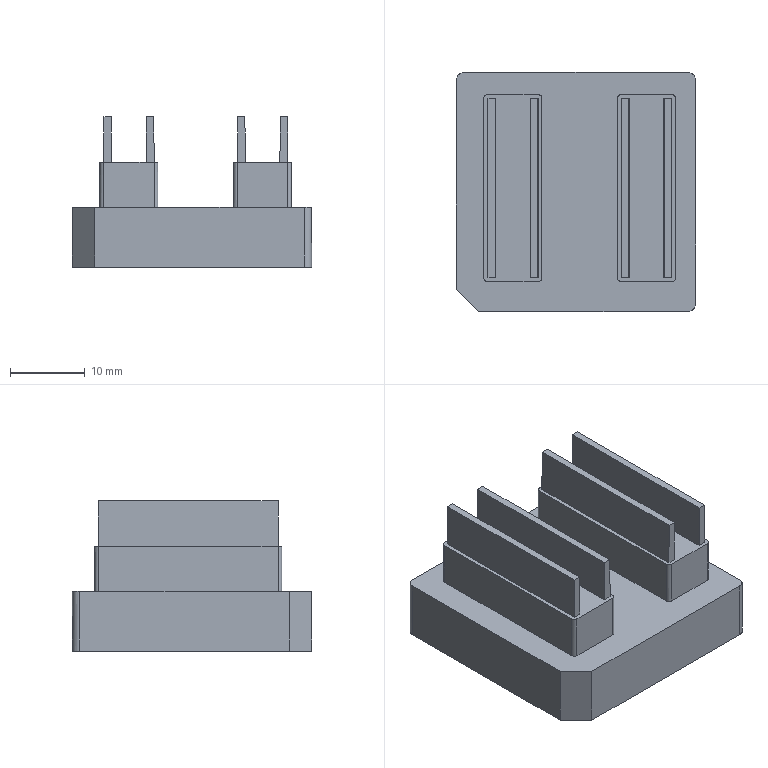NC program | PowerMill | posted with a generic post | part box 32 x 32 x 20.109 mm
Lines 17639 to 18576 of 124326:
N17736 M6
N17737 S8500 M03
N17738 G00 G90 X0.0 Y0.0
N17739 G43 Z11.799 H3
N17740
N17741 G05 P10000 R8
N17742 X15.0099 Y-22.0332
N17743 Z0.9292
N17744 G01 Z-0.2708 F360.0
N17745 X13.9138 Y-16.8733 F600.0
N17746 X13.82 Y17.8929
N17747 X13.5596 Y17.9372
N17748 X13.3468 Y17.9633
N17749 X13.1156 Y17.9827
N17750 X12.8038 Y17.9934
N17751 X11.7079 Y17.9924
N17752 X11.4173 Y17.9789
N17753 X11.2092 Y17.9599
N17754 X11.0271 Y17.9367
N17755 X10.8474 Y17.9075
N17756 X10.562 Y17.8485
N17757 X10.2766 Y17.7734
N17758 X9.9964 Y17.6832
N17759 X9.7057 Y17.5716
N17760 X9.4461 Y17.4547
N17761 X9.3999 Y17.477
N17762 X9.4915 Y-16.4749
N17763 X9.4468 Y-16.4548
N17764 X9.2705 Y-16.5356
N17765 X9.0907 Y-16.6079
N17766 G02 X8.6522 Y-16.7622 I-1.6733 J4.0563
N17767 G01 X8.3857 Y-16.8343
N17768 X8.0819 Y-16.9006
N17769 X7.8594 Y-16.9374
N17770 X7.5105 Y-16.9761
N17771 X7.2257 Y-16.9912
N17772 X6.1649 Y-16.9935
N17773 X5.826 Y-16.9853
N17774 X5.5717 Y-16.9665
N17775 X5.2196 Y-16.9201
N17776 X5.0713 Y-16.892
N17777 X4.9775 Y17.8737
N17778 G00 Z3.9992
N17779 G01 X-3.0555 Y-22.0678 F10000.0
N17780 G00 Z0.9292
N17781 G01 Z-0.2708 F360.0
N17782 X-4.0258 Y-16.8828 F600.0
N17783 X-4.0473 Y17.8862
N17784 X-4.3285 Y17.9368
N17785 G03 X-4.8989 Y17.9892 I-0.8406 J-6.0212
N17786 G01 X-5.2165 Y17.9935
N17787 X-6.2303 Y17.9911
N17788 X-6.5074 Y17.9761
N17789 X-6.8647 Y17.9366
N17790 X-7.0865 Y17.8997
N17791 X-7.3668 Y17.8396
N17792 X-7.6574 Y17.7606
N17793 G03 X-8.4454 Y17.455 I1.6281 J-5.367
N17794 G01 X-8.4559 Y17.4602
N17795 X-8.435 Y-16.4601
N17796 X-8.4457 Y-16.4552
N17797 X-8.711 Y-16.5739
N17798 X-8.9966 Y-16.6831
N17799 X-9.2973 Y-16.779
N17800 X-9.5621 Y-16.8483
N17801 X-9.7937 Y-16.897
N17802 X-10.0271 Y-16.9367
N17803 X-10.2617 Y-16.9654
N17804 X-10.4825 Y-16.9825
N17805 X-10.7037 Y-16.9922
N17806 X-11.8599 Y-16.9928
N17807 X-12.1111 Y-16.983
N17808 X-12.3358 Y-16.9645
N17809 X-12.563 Y-16.9367
N17810 X-12.8437 Y-16.8882
N17811 X-12.8651 Y17.8823
N17812 G00 Z11.799
N17813 G05 P0
N17814 (---------------)
N17815 ( END TOOLPATH : 精公基准台01-平坦面平行-D10 )
N17816 (---------------)
N17817 ( START TOOLPATH : 精公基准台01-基准面偏置-D10 )
N17818 (---------------)
N17819 G00 X0.0 Y0.0 Z9.7992
N17820 G05 P10000 R8
N17821 X26.755 Y-4.9778
N17822 Z-11.11
N17823 G01 Z-12.31 F360.0
N17824 X21.48 F600.0
N17825 X18.7097 Y0.5627
N17826 Y-11.2546
N17827 X18.7014 Y-11.8173
N17828 X18.6806 Y-12.0987
N17829 X18.6457 Y-12.3801
N17830 X18.5701 Y-12.7867
N17831 X18.5333 Y-12.9428
N17832 X18.4555 Y-13.2242
N17833 X18.3621 Y-13.5055
N17834 X18.2525 Y-13.7869
N17835 X18.1258 Y-14.0683
N17836 X18.0074 Y-14.3002
N17837 X17.815 Y-14.631
N17838 X17.6412 Y-14.8938
N17839 X17.415 Y-15.1937
N17840 X17.1741 Y-15.4751
N17841 X17.0423 Y-15.6158
N17842 X16.8819 Y-15.774
N17843 X16.6005 Y-16.0251
N17844 X16.3192 Y-16.2464
N17845 X16.2181 Y-16.3192
N17846 X15.9873 Y-16.4738
N17847 X15.7565 Y-16.6135
N17848 X15.4903 Y-16.7573
N17849 X15.1937 Y-16.8973
N17850 X14.9124 Y-17.0124
N17851 X14.631 Y-17.1108
N17852 X14.3496 Y-17.1933
N17853 X14.0683 Y-17.2616
N17854 X13.7869 Y-17.3151
N17855 X13.5055 Y-17.3545
N17856 X13.2242 Y-17.3791
N17857 X12.9428 Y-17.3924
N17858 X5.9087 Y-17.3915
N17859 X5.6273 Y-17.3773
N17860 X5.3459 Y-17.35
N17861 X5.0646 Y-17.3084
N17862 X4.7832 Y-17.2529
N17863 X4.5018 Y-17.1831
N17864 X4.2205 Y-17.098
N17865 X3.9391 Y-16.997
N17866 X3.663 Y-16.8819
N17867 X3.3764 Y-16.7448
N17868 X3.095 Y-16.5896
N17869 X2.8137 Y-16.4154
N17870 X2.6732 Y-16.3192
N17871 X2.4621 Y-16.1629
N17872 X2.2509 Y-15.9897
N17873 X1.9907 Y-15.7565
N17874 X1.8334 Y-15.5998
N17875 X1.6882 Y-15.4432
N17876 X1.4755 Y-15.1937
N17877 X1.2946 Y-14.9562
N17878 G03 X-0.2981 Y-14.9582 I-0.7956 J-0.6059
N17879 G01 X-0.4765 Y-15.1937
N17880 X-0.5627 Y-15.2976
N17881 X-0.7639 Y-15.5262
N17882 X-0.9908 Y-15.7565
N17883 X-1.1255 Y-15.8812
N17884 X-1.4001 Y-16.1145
N17885 X-1.6882 Y-16.3296
N17886 X-1.9696 Y-16.515
N17887 X-2.2509 Y-16.6783
N17888 X-2.4582 Y-16.7861
N17889 X-2.6625 Y-16.8819
N17890 X-2.8137 Y-16.947
N17891 X-3.095 Y-17.0551
N17892 X-3.3764 Y-17.1471
N17893 X-3.6577 Y-17.2231
N17894 X-3.9391 Y-17.2856
N17895 X-4.2205 Y-17.333
N17896 X-4.5018 Y-17.3663
N17897 X-4.7832 Y-17.3863
N17898 X-5.0646 Y-17.3935
N17899 X-11.8173
N17900 X-12.0987 Y-17.3869
N17901 X-12.3801 Y-17.3677
N17902 X-12.6614 Y-17.3346
N17903 X-12.9428 Y-17.2872
N17904 X-13.2242 Y-17.2259
N17905 X-13.5055 Y-17.1498
N17906 X-13.7869 Y-17.0582
N17907 X-14.0683 Y-16.9509
N17908 X-14.2496 Y-16.8724
N17909 X-14.4284 Y-16.7883
N17910 X-14.631 Y-16.6833
N17911 X-14.9124 Y-16.5204
N17912 X-15.2179 Y-16.3192
N17913 X-15.4872 Y-16.117
N17914 X-15.7565 Y-15.8892
N17915 X-15.9004 Y-15.7565
N17916 X-16.1203 Y-15.5336
N17917 X-16.3192 Y-15.3108
N17918 X-16.4156 Y-15.1937
N17919 X-16.628 Y-14.9124
N17920 X-16.8154 Y-14.631
N17921 X-16.8819 Y-14.5216
N17922 X-17.0104 Y-14.2949
N17923 X-17.1259 Y-14.0683
N17924 X-17.2526 Y-13.7869
N17925 X-17.3622 Y-13.5055
N17926 X-17.4446 Y-13.2591
N17927 X-17.5328 Y-12.9428
N17928 X-17.5967 Y-12.6614
N17929 X-17.6455 Y-12.3801
N17930 X-17.68 Y-12.0987
N17931 X-17.7013 Y-11.8173
N17932 X-17.7098 Y-11.2546
N17933 X-17.7077 Y12.6614
N17934 X-17.6939 Y12.9428
N17935 X-17.6667 Y13.2242
N17936 X-17.6254 Y13.5055
N17937 X-17.5702 Y13.7869
N17938 X-17.5004 Y14.0683
N17939 X-17.4446 Y14.259
N17940 X-17.3152 Y14.631
N17941 X-17.1982 Y14.9124
N17942 X-17.0635 Y15.1937
N17943 X-16.8819 Y15.5204
N17944 X-16.7346 Y15.7565
N17945 X-16.5405 Y16.0325
N17946 X-16.3101 Y16.3192
N17947 X-16.0571 Y16.6005
N17948 X-15.911 Y16.7466
N17949 X-15.7565 Y16.8896
N17950 X-15.4751 Y17.1273
N17951 X-15.1937 Y17.3361
N17952 X-15.0324 Y17.4446
N17953 X-14.8317 Y17.5697
N17954 X-14.631 Y17.6834
N17955 X-14.3496 Y17.8262
N17956 X-14.0683 Y17.9508
N17957 X-13.9251 Y18.0074
N17958 X-13.5055 Y18.1497
N17959 X-13.2242 Y18.2253
N17960 X-12.9428 Y18.2874
N17961 X-12.6614 Y18.3346
N17962 X-12.3801 Y18.3671
N17963 X-12.0987 Y18.3871
N17964 X-11.8173 Y18.3937
N17965 X-5.0646
N17966 X-4.7832 Y18.3867
N17967 X-4.5018 Y18.3671
N17968 X-4.2205 Y18.3332
N17969 X-3.9391 Y18.2854
N17970 X-3.6577 Y18.2235
N17971 X-3.3764 Y18.147
N17972 X-2.9659 Y18.0074
N17973 X-2.8137 Y17.9469
N17974 X-2.5323 Y17.8218
N17975 X-2.2509 Y17.6782
N17976 X-1.8585 Y17.4446
N17977 X-1.6882 Y17.3298
N17978 X-1.4081 Y17.1203
N17979 X-1.1255 Y16.8808
N17980 X-0.98 Y16.7462
N17981 X-0.8331 Y16.5995
N17982 X-0.5627 Y16.2997
N17983 X-0.3183 Y15.9869
N17984 G03 X1.3179 Y15.9858 I0.8185 J0.5745
N17985 G01 X1.3545 Y16.0378
N17986 X1.581 Y16.3192
N17987 X1.6882 Y16.4428
N17988 X1.8941 Y16.6617
N17989 X2.1265 Y16.8819
N17990 X2.2509 Y16.9915
N17991 X2.5323 Y17.2168
N17992 X2.8587 Y17.4446
N17993 X3.1175 Y17.6035
N17994 X3.3764 Y17.7447
N17995 X3.6582 Y17.8799
N17996 X3.966 Y18.0074
N17997 X4.2339 Y18.1024
N17998 X4.5018 Y18.1827
N17999 X4.7832 Y18.2528
N18000 X5.0646 Y18.3085
N18001 X5.3459 Y18.3496
N18002 X5.6273 Y18.3761
N18003 X5.9087 Y18.3917
N18004 X12.9428 Y18.3923
N18005 X13.2242 Y18.3801
N18006 X13.5055 Y18.3547
N18007 X13.7869 Y18.3153
N18008 X14.0683 Y18.2615
N18009 X14.3496 Y18.1939
N18010 X14.631 Y18.111
N18011 X14.9257 Y18.0074
N18012 X15.1937 Y17.8972
N18013 X15.4751 Y17.7651
N18014 X15.7565 Y17.6128
N18015 X16.0326 Y17.4446
N18016 X16.3192 Y17.2463
N18017 X16.5412 Y17.0731
N18018 X16.7646 Y16.8819
N18019 X16.8819 Y16.7742
N18020 X17.1089 Y16.546
N18021 X17.3119 Y16.3192
N18022 X17.4446 Y16.1573
N18023 X17.5971 Y15.9557
N18024 X17.7345 Y15.7565
N18025 X17.8791 Y15.5267
N18026 X18.0074 Y15.3003
N18027 X18.0634 Y15.1937
N18028 X18.1982 Y14.9124
N18029 X18.3151 Y14.631
N18030 X18.4159 Y14.3496
N18031 X18.5003 Y14.0683
N18032 X18.5701 Y13.7863
N18033 X18.6253 Y13.5055
N18034 X18.6665 Y13.2242
N18035 X18.6927 Y12.9428
N18036 X18.7078 Y12.6614
N18037 X18.7097 Y0.5627
N18038 G00 Z9.7992
N18039 G05 P0
N18040 (---------------)
N18041 ( END TOOLPATH : 精公基准台01-基准面偏置-D10 )
N18042 (---------------)
N18043 ( START TOOLPATH : 精公基准台01-外形侧光-D10 )
N18044 (---------------)
N18045 G00 X0.0 Y0.0 Z10.799
N18046 G05 P10000 R8
N18047 X0.5029 Y-13.8692
N18048 Z-11.08
N18049 G01 Z-12.28 F360.0
N18050 G03 X-0.4439 Y-14.5185 I0.3104 J-1.4675 F600.0
N18051 G02 X-5.1116 Y-17.0235 I-4.6196 J3.0068
N18052 G01 X-8.447 Y-17.0234
N18053 X-11.8682 Y-17.0233
N18054 G02 X-17.3397 Y-11.501 I0.0399 J5.5112
N18055 G01 X-17.3393 Y0.4564
N18056 X-17.3389 Y12.5992
N18057 G02 X-11.8662 Y18.0234 I5.5106 J-0.0871
N18058 G01 X-5.1108 Y18.0235
N18059 G02 X0.4478 Y12.5964 I0.047 J-5.512
N18060 G01 X0.4485 Y-11.5023
N18061 G02 X-0.4439 Y-14.5185 I-5.512 J-0.0094
N18062 G03 X-0.6542 Y-15.6471 I1.2572 J-0.8182
N18063 G01 X0.4545 Y-13.781
N18064 G03 X-0.4871 Y-14.4379 I0.3222 J-1.465
N18065 G02 X-5.1116 Y-16.9435 I-4.5764 J2.9262
N18066 G01 X-8.447 Y-16.9434
N18067 X-11.8662
N18068 G02 X-17.2597 Y-11.501 I0.0379 J5.4313
N18069 G01 Y0.4564
N18070 Y12.4138
N18071 G02 X-11.8662 Y17.9434 I5.4334 J0.0955
N18072 G01 X-5.1116 Y17.9435
N18073 G02 X0.3685 Y12.4138 I0.0458 J-5.4349
N18074 G01 Y-11.501
N18075 G02 X-0.4871 Y-14.4379 I-5.432 J-0.0107
N18076 G03 X-0.6883 Y-15.5682 I1.2638 J-0.8081
N18077 G00 Z3.9551
N18078 G01 X18.407 Y-13.8387 F10000.0
N18079 G00 Z-11.08
N18080 G01 Z-12.28 F360.0
N18081 G03 X17.4637 Y-14.4932 I0.3184 J-1.4658 F600.0
N18082 G02 X12.7789 Y-17.0235 I-4.636 J2.9815
N18083 G01 X6.0223 Y-17.0233
N18084 G02 X0.5515 Y-11.501 I0.0406 J5.5112
N18085 G01 X0.5519 Y0.4564
N18086 X0.5523 Y12.5992
N18087 G02 X1.2792 Y15.2491 I5.5107 J-0.0871
N18088 G02 X6.0244 Y18.0234 I4.7837 J-2.737
N18089 G01 X12.7797 Y18.0235
N18090 G02 X18.339 Y12.5964 I0.048 J-5.5118
N18091 G01 X18.3397 Y-11.5023
N18092 G02 X17.4637 Y-14.4932 I-5.512 J-0.0094
N18093 G03 X17.2595 Y-15.6229 I1.2617 J-0.8113
N18094 G01 X18.3581 Y-13.7505
N18095 G03 X17.4202 Y-14.4126 I0.3303 J-1.4632
N18096 G02 X12.7789 Y-16.9435 I-4.5925 J2.9009
N18097 G01 X6.0244 Y-16.9434
N18098 G02 X0.6315 Y-11.501 I0.0385 J5.4313
N18099 G01 Y0.4564
N18100 Y12.4138
N18101 G02 X1.3489 Y15.2092 I5.4334 J0.0955
N18102 G02 X6.0244 Y17.9434 I4.716 J-2.6999
N18103 G01 X12.7789 Y17.9435
N18104 G02 X18.2597 Y12.4138 I0.0469 J-5.4345
N18105 G01 Y-11.501
N18106 G02 X17.4202 Y-14.4126 I-5.432 J-0.0107
N18107 G03 X17.2252 Y-15.544 I1.2682 J-0.8011
N18108 G00 Z10.799
N18109 G05 P0
N18110 (---------------)
N18111 ( END TOOLPATH : 精公基准台01-外形侧光-D10 )
N18112 (---------------)
N18113 ( START TOOLPATH : 精公基准台01-基准台侧光-D10 )
N18114 (---------------)
N18115 G00 X0.0 Y0.0 Z9.7992
N18116 G05 P10000 R8
N18117 X21.439 Y-24.0159
N18118 Z-19.01
N18119 G01 Z-20.21 F360.0
N18120 G03 X18.4869 Y-19.9804 I-1.476 J2.0177 F600.0
N18121 G01 X18.4851 Y-19.9817
N18122 X18.4839 Y-19.9826
N18123 X18.4827 Y-19.9835
N18124 X18.3812 Y-20.052
N18125 X18.3801 Y-20.0527
N18126 X18.379 Y-20.0535
N18127 X18.0629 Y-20.2521
N18128 X18.0607 Y-20.2534
N18129 X18.0585 Y-20.2547
N18130 X17.7423 Y-20.4263
N18131 X17.7402 Y-20.4274
N18132 X17.7381 Y-20.4285
N18133 X17.422 Y-20.5767
N18134 X17.4199 Y-20.5776
N18135 X17.4178 Y-20.5785
N18136 X17.1016 Y-20.7052
N18137 X17.0995 Y-20.706
N18138 X17.0974 Y-20.7067
N18139 X16.7812 Y-20.8131
N18140 X16.7791 Y-20.8138
N18141 X16.777 Y-20.8144
N18142 X16.4609 Y-20.9018
N18143 X16.4593 Y-20.9022
N18144 X16.4576 Y-20.9026
N18145 X16.2808 Y-20.9435
N18146 X16.2797 Y-20.9438
N18147 X16.2785 Y-20.944
N18148 X16.1392 Y-20.9721
N18149 X16.1378 Y-20.9723
N18150 X16.1364 Y-20.9726
N18151 X15.8202 Y-21.0244
N18152 X15.8181 Y-21.0247
N18153 X15.8159 Y-21.025
N18154 X15.4997 Y-21.0591
N18155 X15.4976 Y-21.0593
N18156 X15.4955 Y-21.0595
N18157 X15.1794 Y-21.0768
N18158 X15.1776 Y-21.0769
N18159 X15.1758
N18160 X14.8596 Y-21.08
N18161 X14.8592
N18162 X14.8588
N18163 X-12.962
N18164 X-12.963
N18165 X-12.9639
N18166 X-13.2801 Y-21.0722
N18167 X-13.2826 Y-21.0721
N18168 X-13.2851 Y-21.072
N18169 X-13.6012 Y-21.0443
N18170 X-13.6038 Y-21.044
N18171 X-13.6063 Y-21.0436
N18172 X-13.9224 Y-20.9955
N18173 X-13.925 Y-20.9951
N18174 X-13.9275 Y-20.9946
N18175 X-14.2437 Y-20.9254
N18176 X-14.2462 Y-20.9248
N18177 X-14.2487 Y-20.9241
N18178 X-14.5649 Y-20.8329
N18179 X-14.5674 Y-20.8322
N18180 X-14.5699 Y-20.8313
N18181 X-14.8861 Y-20.7169
N18182 X-14.8882 Y-20.7161
N18183 X-14.8903 Y-20.7152
N18184 X-15.1057 Y-20.623
N18185 X-15.107 Y-20.6225
N18186 X-15.1082 Y-20.6219
N18187 X-15.209 Y-20.5746
N18188 X-15.2107 Y-20.5738
N18189 X-15.2123 Y-20.5729
N18190 X-15.5285 Y-20.406
N18191 X-15.5304 Y-20.4049
N18192 X-15.5324 Y-20.4038
N18193 X-15.7019 Y-20.3019
N18194 X-15.7031 Y-20.3011
N18195 X-15.7044 Y-20.3003
N18196 X-15.851 Y-20.2045
N18197 X-15.8529 Y-20.2033
N18198 X-15.8546 Y-20.202
N18199 X-16.1547 Y-19.9817
N18200 X-16.1573 Y-19.9797
N18201 X-16.1598 Y-19.9776
N18202 X-16.492 Y-19.6894
N18203 X-16.494 Y-19.6876
N18204 X-16.4959 Y-19.6858
N18205 X-16.8121 Y-19.3722
N18206 X-16.8122 Y-19.372
N18207 X-16.8123 Y-19.3719
N18208 X-19.6576 Y-16.5254
N18209 X-19.6594 Y-16.5235
N18210 X-19.6611 Y-16.5216
N18211 X-19.9645 Y-16.1762
N18212 X-19.9667 Y-16.1736
N18213 X-19.9688 Y-16.1709
N18214 X-20.2019 Y-15.8548
N18215 X-20.2032 Y-15.8529
N18216 X-20.2045 Y-15.851
N18217 X-20.3003 Y-15.7044
N18218 X-20.3011 Y-15.7031
N18219 X-20.3019 Y-15.7019
N18220 X-20.4038 Y-15.5324
N18221 X-20.4049 Y-15.5304
N18222 X-20.406 Y-15.5285
N18223 X-20.5729 Y-15.2123
N18224 X-20.5738 Y-15.2107
N18225 X-20.5746 Y-15.209
N18226 X-20.6219 Y-15.1082
N18227 X-20.6225 Y-15.107
N18228 X-20.623 Y-15.1057
N18229 X-20.7152 Y-14.8903
N18230 X-20.7161 Y-14.8882
N18231 X-20.7169 Y-14.8861
N18232 X-20.8313 Y-14.5699
N18233 X-20.8322 Y-14.5674
N18234 X-20.8329 Y-14.5649
N18235 X-20.9241 Y-14.2487
N18236 X-20.9248 Y-14.2462
N18237 X-20.9254 Y-14.2437
N18238 X-20.9946 Y-13.9275
N18239 X-20.9951 Y-13.925
N18240 X-20.9955 Y-13.9224
N18241 X-21.0436 Y-13.6063
N18242 X-21.044 Y-13.6038
N18243 X-21.0443 Y-13.6012
N18244 X-21.072 Y-13.2851
N18245 X-21.0721 Y-13.2826
N18246 X-21.0722 Y-13.2801
N18247 X-21.08 Y-12.9639
N18248 Y-12.963
N18249 Y-12.962
N18250 Y14.8588
N18251 Y14.8592
N18252 Y14.8596
N18253 X-21.077 Y15.1758
N18254 X-21.0769 Y15.1775
N18255 X-21.0768 Y15.1793
N18256 X-21.0597 Y15.4955
N18257 X-21.0596 Y15.4976
N18258 X-21.0594 Y15.4998
N18259 X-21.025 Y15.8159
N18260 X-21.0247 Y15.8181
N18261 X-21.0244 Y15.8202
N18262 X-20.9728 Y16.1363
N18263 X-20.9724 Y16.1384
N18264 X-20.972 Y16.1405
N18265 X-20.9029 Y16.4567
N18266 X-20.9024 Y16.4588
N18267 X-20.9018 Y16.4609
N18268 X-20.8145 Y16.777
N18269 X-20.8139 Y16.7792
N18270 X-20.8131 Y16.7814
N18271 X-20.706 Y17.0975
N18272 X-20.7053 Y17.0995
N18273 X-20.7046 Y17.1015
N18274 X-20.5786 Y17.4176
N18275 X-20.5776 Y17.4199
N18276 X-20.5766 Y17.4221
N18277 X-20.4277 Y17.7383
N18278 X-20.4267 Y17.7402
N18279 X-20.4257 Y17.7422
N18280 X-20.2547 Y18.0584
N18281 X-20.2535 Y18.0605
N18282 X-20.2522 Y18.0627
N18283 X-20.0546 Y18.3788
N18284 X-20.0537 Y18.3802
N18285 X-20.0528 Y18.3816
N18286 X-19.9832 Y18.4834
N18287 X-19.9825 Y18.4845
N18288 X-19.9817 Y18.4855
N18289 X-19.8246 Y18.6999
N18290 X-19.8236 Y18.7013
N18291 X-19.8225 Y18.7026
N18292 X-19.6635 Y18.9011
N18293 X-19.6626 Y18.9021
N18294 X-19.6617 Y18.9032
N18295 X-19.5606 Y19.0209
N18296 X-19.5595 Y19.0221
N18297 X-19.5585 Y19.0232
N18298 X-19.3435 Y19.2544
N18299 X-19.3425 Y19.2554
N18300 X-19.3415 Y19.2565
N18301 X-19.2565 Y19.3415
N18302 X-19.2554 Y19.3425
N18303 X-19.2544 Y19.3435
N18304 X-19.0232 Y19.5584
N18305 X-19.022 Y19.5596
N18306 X-19.0207 Y19.5607
N18307 X-18.9022 Y19.6619
N18308 X-18.9013 Y19.6626
N18309 X-18.9004 Y19.6634
N18310 X-18.7028 Y19.8224
N18311 X-18.7013 Y19.8236
N18312 X-18.6998 Y19.8247
N18313 X-18.4851 Y19.9817
N18314 X-18.4839 Y19.9826
N18315 X-18.4827 Y19.9835
N18316 X-18.3812 Y20.052
N18317 X-18.3801 Y20.0527
N18318 X-18.379 Y20.0535
N18319 X-18.0629 Y20.2521
N18320 X-18.0607 Y20.2534
N18321 X-18.0585 Y20.2547
N18322 X-17.7423 Y20.4263
N18323 X-17.7402 Y20.4274
N18324 X-17.7381 Y20.4285
N18325 X-17.422 Y20.5767
N18326 X-17.4199 Y20.5776
N18327 X-17.4178 Y20.5785
N18328 X-17.1016 Y20.7052
N18329 X-17.0995 Y20.706
N18330 X-17.0974 Y20.7067
N18331 X-16.7812 Y20.8131
N18332 X-16.7791 Y20.8138
N18333 X-16.777 Y20.8144
N18334 X-16.4609 Y20.9018
N18335 X-16.4588 Y20.9023
N18336 X-16.4566 Y20.9028
N18337 X-16.1405 Y20.9718
N18338 X-16.1384 Y20.9722
N18339 X-16.1364 Y20.9726
N18340 X-15.8202 Y21.0244
N18341 X-15.8181 Y21.0247
N18342 X-15.8159 Y21.025
N18343 X-15.4997 Y21.0591
N18344 X-15.4976 Y21.0593
N18345 X-15.4955 Y21.0595
N18346 X-15.1794 Y21.0768
N18347 X-15.1776 Y21.0769
N18348 X-15.1758
N18349 X-14.8596 Y21.08
N18350 X-14.8592
N18351 X-14.8588
N18352 X14.8588
N18353 X14.8592
N18354 X14.8596
N18355 X15.1758 Y21.077
N18356 X15.1775 Y21.0769
N18357 X15.1793 Y21.0768
N18358 X15.4955 Y21.0597
N18359 X15.4976 Y21.0596
N18360 X15.4998 Y21.0594
N18361 X15.8159 Y21.025
N18362 X15.8181 Y21.0247
N18363 X15.8202 Y21.0244
N18364 X16.1363 Y20.9728
N18365 X16.1384 Y20.9724
N18366 X16.1405 Y20.972
N18367 X16.4567 Y20.9029
N18368 X16.4588 Y20.9024
N18369 X16.4609 Y20.9018
N18370 X16.777 Y20.8145
N18371 X16.7792 Y20.8139
N18372 X16.7814 Y20.8132
N18373 X17.0975 Y20.7061
N18374 X17.0995 Y20.7054
N18375 X17.1015 Y20.7046
N18376 X17.4176 Y20.5786
N18377 X17.4199 Y20.5776
N18378 X17.4221 Y20.5766
N18379 X17.7382 Y20.4277
N18380 X17.7402 Y20.4267
N18381 X17.7422 Y20.4257
N18382 X18.0584 Y20.2547
N18383 X18.0605 Y20.2535
N18384 X18.0627 Y20.2522
N18385 X18.3788 Y20.0546
N18386 X18.3802 Y20.0537
N18387 X18.3816 Y20.0528
N18388 X18.4834 Y19.9832
N18389 X18.4845 Y19.9825
N18390 X18.4855 Y19.9817
N18391 X18.6999 Y19.8246
N18392 X18.7013 Y19.8236
N18393 X18.7026 Y19.8225
N18394 X18.9011 Y19.6635
N18395 X18.9021 Y19.6626
N18396 X18.9032 Y19.6617
N18397 X19.0209 Y19.5606
N18398 X19.0221 Y19.5595
N18399 X19.0232 Y19.5585
N18400 X19.2544 Y19.3435
N18401 X19.2554 Y19.3425
N18402 X19.2565 Y19.3415
N18403 X19.3415 Y19.2565
N18404 X19.3425 Y19.2554
N18405 X19.3435 Y19.2544
N18406 X19.5584 Y19.0232
N18407 X19.5596 Y19.022
N18408 X19.5607 Y19.0207
N18409 X19.6619 Y18.9022
N18410 X19.6626 Y18.9013
N18411 X19.6634 Y18.9004
N18412 X19.8224 Y18.7028
N18413 X19.8236 Y18.7013
N18414 X19.8247 Y18.6998
N18415 X19.9817 Y18.4851
N18416 X19.9826 Y18.4839
N18417 X19.9835 Y18.4827
N18418 X20.052 Y18.3812
N18419 X20.0527 Y18.3801
N18420 X20.0535 Y18.379
N18421 X20.2521 Y18.0629
N18422 X20.2534 Y18.0607
N18423 X20.2547 Y18.0585
N18424 X20.4263 Y17.7423
N18425 X20.4274 Y17.7402
N18426 X20.4285 Y17.7381
N18427 X20.5767 Y17.422
N18428 X20.5776 Y17.4199
N18429 X20.5785 Y17.4178
N18430 X20.7052 Y17.1016
N18431 X20.706 Y17.0995
N18432 X20.7067 Y17.0974
N18433 X20.8132 Y16.7812
N18434 X20.8138 Y16.7791
N18435 X20.8145 Y16.777
N18436 X20.9018 Y16.4609
N18437 X20.9023 Y16.4588
N18438 X20.9028 Y16.4566
N18439 X20.9718 Y16.1405
N18440 X20.9722 Y16.1384
N18441 X20.9726 Y16.1364
N18442 X21.0244 Y15.8202
N18443 X21.0247 Y15.8181
N18444 X21.025 Y15.8159
N18445 X21.0591 Y15.4997
N18446 X21.0593 Y15.4976
N18447 X21.0595 Y15.4955
N18448 X21.0768 Y15.1794
N18449 X21.0769 Y15.1776
N18450 Y15.1758
N18451 X21.08 Y14.8596
N18452 Y14.8592
N18453 Y14.8588
N18454 Y0.0
N18455 Y-14.8588
N18456 Y-14.8592
N18457 Y-14.8596
N18458 X21.0769 Y-15.1758
N18459 Y-15.1775
N18460 X21.0768 Y-15.1793
N18461 X21.0597 Y-15.4955
N18462 X21.0596 Y-15.4976
N18463 X21.0594 Y-15.4998
N18464 X21.025 Y-15.8159
N18465 X21.0247 Y-15.8181
N18466 X21.0244 Y-15.8202
N18467 X20.9728 Y-16.1363
N18468 X20.9724 Y-16.1384
N18469 X20.972 Y-16.1405
N18470 X20.9029 Y-16.4567
N18471 X20.9024 Y-16.4588
N18472 X20.9018 Y-16.4609
N18473 X20.8145 Y-16.777
N18474 X20.8139 Y-16.7792
N18475 X20.8131 Y-16.7814
N18476 X20.706 Y-17.0975
N18477 X20.7053 Y-17.0995
N18478 X20.7046 Y-17.1015
N18479 X20.5786 Y-17.4176
N18480 X20.5776 Y-17.4199
N18481 X20.5766 Y-17.4221
N18482 X20.4277 Y-17.7383
N18483 X20.4267 Y-17.7402
N18484 X20.4257 Y-17.7422
N18485 X20.2547 Y-18.0584
N18486 X20.2535 Y-18.0605
N18487 X20.2522 Y-18.0627
N18488 X20.0546 Y-18.3788
N18489 X20.0537 Y-18.3802
N18490 X20.0528 Y-18.3816
N18491 X19.9832 Y-18.4834
N18492 X19.9825 Y-18.4845
N18493 X19.9817 Y-18.4855
N18494 X19.8246 Y-18.6999
N18495 X19.8236 Y-18.7013
N18496 X19.8225 Y-18.7026
N18497 X19.6635 Y-18.9011
N18498 X19.6626 Y-18.9021
N18499 X19.6617 Y-18.9032
N18500 X19.5606 Y-19.0209
N18501 X19.5595 Y-19.0221
N18502 X19.5585 Y-19.0232
N18503 X19.3435 Y-19.2544
N18504 X19.3425 Y-19.2554
N18505 X19.3415 Y-19.2565
N18506 X19.2565 Y-19.3415
N18507 X19.2554 Y-19.3425
N18508 X19.2544 Y-19.3435
N18509 X19.0232 Y-19.5584
N18510 X19.022 Y-19.5596
N18511 X19.0207 Y-19.5607
N18512 X18.9022 Y-19.6619
N18513 X18.9013 Y-19.6626
N18514 X18.9004 Y-19.6634
N18515 X18.7028 Y-19.8224
N18516 X18.7013 Y-19.8236
N18517 X18.6998 Y-19.8247
N18518 X18.4869 Y-19.9804
N18519 G03 X21.439 Y-24.0159 I1.4761 J-2.0178
N18520 G01 X21.2354 Y-24.0613
N18521 G03 X18.4356 Y-19.9187 I-1.3999 J2.0713
N18522 G01 X18.3364 Y-19.9857
N18523 X18.0203 Y-20.1844
N18524 X17.7042 Y-20.356
N18525 X17.388 Y-20.5043
N18526 X17.0719 Y-20.6309
N18527 X16.7557 Y-20.7373
N18528 X16.4396 Y-20.8246
N18529 X16.2628 Y-20.8656
N18530 X16.1234 Y-20.8936
N18531 X15.8073 Y-20.9454
N18532 X15.4911 Y-20.9796
N18533 X15.175 Y-20.9969
N18534 X14.8588 Y-21.0
N18535 X-12.962
N18536 X-13.2781 Y-20.9923
N18537 X-13.5943 Y-20.9646
N18538 X-13.9104 Y-20.9164
N18539 X-14.2266 Y-20.8472
N18540 X-14.5427 Y-20.7561
N18541 X-14.8588 Y-20.6416
N18542 X-15.0742 Y-20.5495
N18543 X-15.175 Y-20.5022
N18544 X-15.4911 Y-20.3352
N18545 X-15.6607 Y-20.2333
N18546 X-15.8073 Y-20.1375
N18547 X-16.1074 Y-19.9172
N18548 X-16.4396 Y-19.629
N18549 X-16.7557 Y-19.3154
N18550 X-19.2849 Y-16.7862
N18551 X-19.601 Y-16.4688
N18552 X-19.9044 Y-16.1234
N18553 X-20.1375 Y-15.8073
N18554 X-20.2333 Y-15.6607
N18555 X-20.3352 Y-15.4911
N18556 X-20.5022 Y-15.175
N18557 X-20.5495 Y-15.0742
N18558 X-20.6416 Y-14.8588
N18559 X-20.7561 Y-14.5427
N18560 X-20.8472 Y-14.2266
N18561 X-20.9164 Y-13.9104
N18562 X-20.9646 Y-13.5943
N18563 X-20.9923 Y-13.2781
N18564 X-21.0 Y-12.962
N18565 Y14.8588
N18566 X-20.997 Y15.175
N18567 X-20.9799 Y15.4911
N18568 X-20.9454 Y15.8073
N18569 X-20.8939 Y16.1234
N18570 X-20.8247 Y16.4396
N18571 X-20.7374 Y16.7557
N18572 X-20.6303 Y17.0719
N18573 X-20.5043 Y17.388
N18574 X-20.3553 Y17.7042
N18575 X-20.1844 Y18.0203
N18576 X-19.9868 Y18.3364
N18577 X-19.9172 Y18.4382
N18578 X-19.7601 Y18.6526
N18579 X-19.601 Y18.851
N18580 X-19.4999 Y18.9687
N18581 X-19.2849 Y19.1999
N18582 X-19.1999 Y19.2849
N18583 X-18.9687 Y19.4998
N18584 X-18.8502 Y19.601
N18585 X-18.6526 Y19.7601
N18586 X-18.4379 Y19.9172
N18587 X-18.3364 Y19.9857
N18588 X-18.0203 Y20.1844
N18589 X-17.7042 Y20.356
N18590 X-17.388 Y20.5043
N18591 X-17.0719 Y20.6309
N18592 X-16.7557 Y20.7373
N18593 X-16.4396 Y20.8246
N18594 X-16.1234 Y20.8936
N18595 X-15.8073 Y20.9454
N18596 X-15.4911 Y20.9796
N18597 X-15.175 Y20.997
N18598 X-14.8588 Y21.0
N18599 X14.8588
N18600 X15.175 Y20.997
N18601 X15.4911 Y20.9799
N18602 X15.8073 Y20.9454
N18603 X16.1234 Y20.8939
N18604 X16.4396 Y20.8247
N18605 X16.7557 Y20.7374
N18606 X17.0719 Y20.6303
N18607 X17.388 Y20.5043
N18608 X17.7042 Y20.3553
N18609 X18.0203 Y20.1844
N18610 X18.3364 Y19.9868
N18611 X18.4382 Y19.9172
N18612 X18.6526 Y19.7601
N18613 X18.851 Y19.601
N18614 X18.9687 Y19.4999
N18615 X19.1999 Y19.2849
N18616 X19.2849 Y19.1999
N18617 X19.4998 Y18.9687
N18618 X19.601 Y18.8502
N18619 X19.7601 Y18.6526
N18620 X19.9172 Y18.4379
N18621 X19.9857 Y18.3364
N18622 X20.1844 Y18.0203
N18623 X20.356 Y17.7042
N18624 X20.5043 Y17.388
N18625 X20.6309 Y17.0719
N18626 X20.7373 Y16.7557
N18627 X20.8246 Y16.4396
N18628 X20.8936 Y16.1234
N18629 X20.9454 Y15.8073
N18630 X20.9796 Y15.4911
N18631 X20.9969 Y15.175
N18632 X21.0 Y14.8588
N18633 Y0.0
N18634 Y-14.8588
N18635 X20.997 Y-15.175
N18636 X20.9799 Y-15.4911
N18637 X20.9454 Y-15.8073
N18638 X20.8938 Y-16.1234
N18639 X20.8247 Y-16.4396
N18640 X20.7374 Y-16.7557
N18641 X20.6303 Y-17.0719
N18642 X20.5043 Y-17.388
N18643 X20.3553 Y-17.7042
N18644 X20.1844 Y-18.0203
N18645 X19.9868 Y-18.3364
N18646 X19.9172 Y-18.4382
N18647 X19.7601 Y-18.6526
N18648 X19.601 Y-18.851
N18649 X19.4999 Y-18.9687
N18650 X19.2849 Y-19.1999
N18651 X19.1999 Y-19.2849
N18652 X18.9687 Y-19.4998
N18653 X18.8502 Y-19.601
N18654 X18.6526 Y-19.7601
N18655 X18.4379 Y-19.9172
N18656 X18.4356 Y-19.9187
N18657 G03 X21.2351 Y-24.0615 I1.3998 J-2.0714
N18658 G00 Z9.7992
N18659 G05 P0
N18660 (---------------)
N18661 ( END TOOLPATH : 精公基准台01-基准台侧光-D10 )
N18662 (---------------)
N18663
N18664 M05
N18665 G53 Z0.0
N18666 (---------------)
N18667 ( START TOOLPATH : 精公精光01-等高-D3 )
N18668 (---------------)
N18669 ( TOOL NO.    :10 )
N18670 ( TOOL TYPE   : ENDMILL)
N18671 ( TOOL ID     : D3_2_1)
N18672 ( TOOL DIA    : 3.0 LENGTH 61.32)
N18673 T10